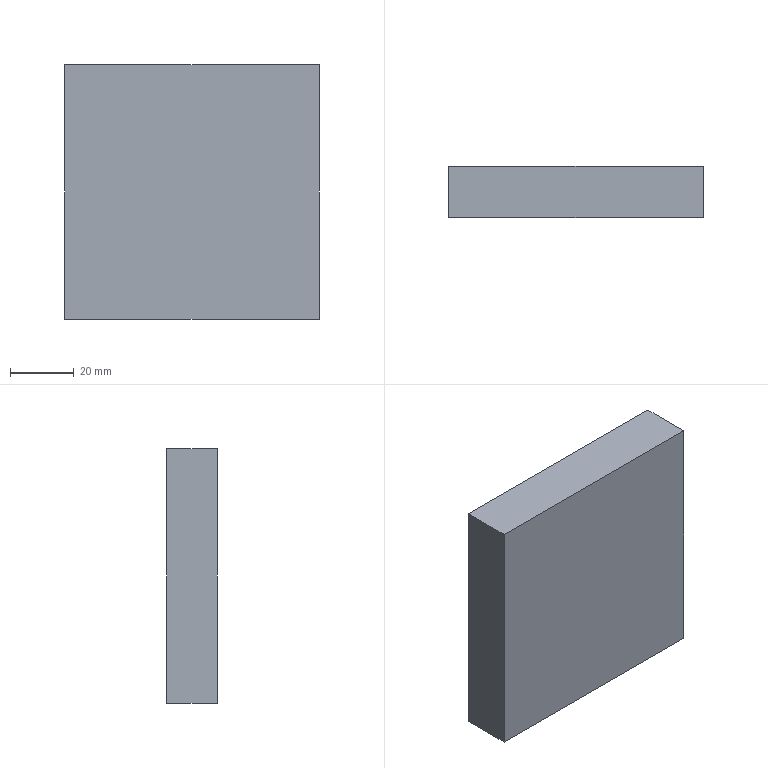Part | STEP file | HXGR200008-05-27 | 1 solid | 8 faces | box 80 x 16 x 80 mm | volume 101387 mm3 | plane 6 | cone 2
STEP:
#1=CARTESIAN_POINT('',(0.,8.008,0.));
#2=VERTEX_POINT('',#1);
#3=CARTESIAN_POINT('',(-11.,16.,0.));
#4=VERTEX_POINT('',#3);
#5=CARTESIAN_POINT('',(-11.,16.,0.));
#6=DIRECTION('',(-0.809,0.5878,0.));
#7=VECTOR('',#6,1000.);
#8=LINE('',#5,#7);
#9=EDGE_CURVE('',#2,#4,#8,.T.);
#10=ORIENTED_EDGE('',*,*,#9,.F.);
#11=CARTESIAN_POINT('',(11.,16.,0.));
#12=VERTEX_POINT('',#11);
#13=CARTESIAN_POINT('',(11.,16.,0.));
#14=DIRECTION('',(0.809,0.5878,0.));
#15=VECTOR('',#14,1000.);
#16=LINE('',#13,#15);
#17=EDGE_CURVE('',#2,#12,#16,.T.);
#18=ORIENTED_EDGE('',*,*,#17,.T.);
#19=CARTESIAN_POINT('',(0.,16.,0.));
#20=DIRECTION('',(0.,1.,0.));
#21=DIRECTION('',(-1.,0.,0.));
#22=AXIS2_PLACEMENT_3D('',#19,#20,#21);
#23=CIRCLE('',#22,11.);
#24=EDGE_CURVE('',#12,#4,#23,.T.);
#25=ORIENTED_EDGE('',*,*,#24,.T.);
#26=EDGE_LOOP('',(#10,#18,#25));
#27=FACE_OUTER_BOUND('',#26,.T.);
#28=CARTESIAN_POINT('',(0.,16.,0.));
#29=DIRECTION('',(0.,1.,0.));
#30=DIRECTION('',(-1.,0.,0.));
#31=AXIS2_PLACEMENT_3D('',#28,#29,#30);
#32=CONICAL_SURFACE('',#31,11.,0.9425);
#33=ADVANCED_FACE('',(#27),#32,.F.);
#34=CARTESIAN_POINT('',(-40.,0.,-40.));
#35=VERTEX_POINT('',#34);
#36=CARTESIAN_POINT('',(-40.,0.,40.));
#37=VERTEX_POINT('',#36);
#38=CARTESIAN_POINT('',(-40.,0.,40.));
#39=DIRECTION('',(0.,0.,1.));
#40=VECTOR('',#39,1000.);
#41=LINE('',#38,#40);
#42=EDGE_CURVE('',#35,#37,#41,.T.);
#43=ORIENTED_EDGE('',*,*,#42,.T.);
#44=CARTESIAN_POINT('',(-40.,16.,40.));
#45=VERTEX_POINT('',#44);
#46=CARTESIAN_POINT('',(-40.,16.,40.));
#47=DIRECTION('',(0.,-1.,0.));
#48=VECTOR('',#47,1000.);
#49=LINE('',#46,#48);
#50=EDGE_CURVE('',#45,#37,#49,.T.);
#51=ORIENTED_EDGE('',*,*,#50,.F.);
#52=CARTESIAN_POINT('',(-40.,16.,-40.));
#53=VERTEX_POINT('',#52);
#54=CARTESIAN_POINT('',(-40.,16.,40.));
#55=DIRECTION('',(0.,0.,1.));
#56=VECTOR('',#55,1000.);
#57=LINE('',#54,#56);
#58=EDGE_CURVE('',#53,#45,#57,.T.);
#59=ORIENTED_EDGE('',*,*,#58,.F.);
#60=CARTESIAN_POINT('',(-40.,16.,-40.));
#61=DIRECTION('',(0.,-1.,0.));
#62=VECTOR('',#61,1000.);
#63=LINE('',#60,#62);
#64=EDGE_CURVE('',#53,#35,#63,.T.);
#65=ORIENTED_EDGE('',*,*,#64,.T.);
#66=EDGE_LOOP('',(#43,#51,#59,#65));
#67=FACE_OUTER_BOUND('',#66,.T.);
#68=CARTESIAN_POINT('',(-40.,16.,40.));
#69=DIRECTION('',(1.,0.,0.));
#70=DIRECTION('',(0.,0.,-1.));
#71=AXIS2_PLACEMENT_3D('',#68,#69,#70);
#72=PLANE('',#71);
#73=ADVANCED_FACE('',(#67),#72,.F.);
#74=CARTESIAN_POINT('',(40.,0.,40.));
#75=VERTEX_POINT('',#74);
#76=CARTESIAN_POINT('',(40.,0.,40.));
#77=DIRECTION('',(1.,0.,0.));
#78=VECTOR('',#77,1000.);
#79=LINE('',#76,#78);
#80=EDGE_CURVE('',#37,#75,#79,.T.);
#81=ORIENTED_EDGE('',*,*,#80,.T.);
#82=CARTESIAN_POINT('',(40.,16.,40.));
#83=VERTEX_POINT('',#82);
#84=CARTESIAN_POINT('',(40.,16.,40.));
#85=DIRECTION('',(0.,-1.,0.));
#86=VECTOR('',#85,1000.);
#87=LINE('',#84,#86);
#88=EDGE_CURVE('',#83,#75,#87,.T.);
#89=ORIENTED_EDGE('',*,*,#88,.F.);
#90=CARTESIAN_POINT('',(40.,16.,40.));
#91=DIRECTION('',(1.,0.,0.));
#92=VECTOR('',#91,1000.);
#93=LINE('',#90,#92);
#94=EDGE_CURVE('',#45,#83,#93,.T.);
#95=ORIENTED_EDGE('',*,*,#94,.F.);
#96=ORIENTED_EDGE('',*,*,#50,.T.);
#97=EDGE_LOOP('',(#81,#89,#95,#96));
#98=FACE_OUTER_BOUND('',#97,.T.);
#99=CARTESIAN_POINT('',(40.,16.,40.));
#100=DIRECTION('',(0.,0.,-1.));
#101=DIRECTION('',(-1.,0.,0.));
#102=AXIS2_PLACEMENT_3D('',#99,#100,#101);
#103=PLANE('',#102);
#104=ADVANCED_FACE('',(#98),#103,.F.);
#105=CARTESIAN_POINT('',(40.,0.,-40.));
#106=VERTEX_POINT('',#105);
#107=CARTESIAN_POINT('',(40.,0.,40.));
#108=DIRECTION('',(0.,0.,-1.));
#109=VECTOR('',#108,1000.);
#110=LINE('',#107,#109);
#111=EDGE_CURVE('',#75,#106,#110,.T.);
#112=ORIENTED_EDGE('',*,*,#111,.T.);
#113=CARTESIAN_POINT('',(40.,16.,-40.));
#114=VERTEX_POINT('',#113);
#115=CARTESIAN_POINT('',(40.,16.,-40.));
#116=DIRECTION('',(0.,-1.,0.));
#117=VECTOR('',#116,1000.);
#118=LINE('',#115,#117);
#119=EDGE_CURVE('',#114,#106,#118,.T.);
#120=ORIENTED_EDGE('',*,*,#119,.F.);
#121=CARTESIAN_POINT('',(40.,16.,40.));
#122=DIRECTION('',(0.,0.,-1.));
#123=VECTOR('',#122,1000.);
#124=LINE('',#121,#123);
#125=EDGE_CURVE('',#83,#114,#124,.T.);
#126=ORIENTED_EDGE('',*,*,#125,.F.);
#127=ORIENTED_EDGE('',*,*,#88,.T.);
#128=EDGE_LOOP('',(#112,#120,#126,#127));
#129=FACE_OUTER_BOUND('',#128,.T.);
#130=CARTESIAN_POINT('',(40.,16.,40.));
#131=DIRECTION('',(-1.,0.,0.));
#132=DIRECTION('',(0.,0.,1.));
#133=AXIS2_PLACEMENT_3D('',#130,#131,#132);
#134=PLANE('',#133);
#135=ADVANCED_FACE('',(#129),#134,.F.);
#136=CARTESIAN_POINT('',(40.,0.,-40.));
#137=DIRECTION('',(-1.,0.,0.));
#138=VECTOR('',#137,1000.);
#139=LINE('',#136,#138);
#140=EDGE_CURVE('',#106,#35,#139,.T.);
#141=ORIENTED_EDGE('',*,*,#140,.T.);
#142=ORIENTED_EDGE('',*,*,#64,.F.);
#143=CARTESIAN_POINT('',(40.,16.,-40.));
#144=DIRECTION('',(-1.,0.,0.));
#145=VECTOR('',#144,1000.);
#146=LINE('',#143,#145);
#147=EDGE_CURVE('',#114,#53,#146,.T.);
#148=ORIENTED_EDGE('',*,*,#147,.F.);
#149=ORIENTED_EDGE('',*,*,#119,.T.);
#150=EDGE_LOOP('',(#141,#142,#148,#149));
#151=FACE_OUTER_BOUND('',#150,.T.);
#152=CARTESIAN_POINT('',(40.,16.,-40.));
#153=DIRECTION('',(0.,0.,1.));
#154=DIRECTION('',(1.,0.,0.));
#155=AXIS2_PLACEMENT_3D('',#152,#153,#154);
#156=PLANE('',#155);
#157=ADVANCED_FACE('',(#151),#156,.F.);
#158=CARTESIAN_POINT('',(0.,16.,0.));
#159=DIRECTION('',(0.,1.,0.));
#160=DIRECTION('',(-1.,0.,0.));
#161=AXIS2_PLACEMENT_3D('',#158,#159,#160);
#162=CIRCLE('',#161,11.);
#163=EDGE_CURVE('',#4,#12,#162,.T.);
#164=ORIENTED_EDGE('',*,*,#163,.F.);
#165=ORIENTED_EDGE('',*,*,#24,.F.);
#166=EDGE_LOOP('',(#164,#165));
#167=FACE_BOUND('',#166,.T.);
#168=ORIENTED_EDGE('',*,*,#58,.T.);
#169=ORIENTED_EDGE('',*,*,#94,.T.);
#170=ORIENTED_EDGE('',*,*,#125,.T.);
#171=ORIENTED_EDGE('',*,*,#147,.T.);
#172=EDGE_LOOP('',(#168,#169,#170,#171));
#173=FACE_OUTER_BOUND('',#172,.T.);
#174=CARTESIAN_POINT('',(0.,16.,0.));
#175=DIRECTION('',(0.,1.,0.));
#176=DIRECTION('',(0.,0.,1.));
#177=AXIS2_PLACEMENT_3D('',#174,#175,#176);
#178=PLANE('',#177);
#179=ADVANCED_FACE('',(#167,#173),#178,.T.);
#180=ORIENTED_EDGE('',*,*,#42,.F.);
#181=ORIENTED_EDGE('',*,*,#140,.F.);
#182=ORIENTED_EDGE('',*,*,#111,.F.);
#183=ORIENTED_EDGE('',*,*,#80,.F.);
#184=EDGE_LOOP('',(#180,#181,#182,#183));
#185=FACE_OUTER_BOUND('',#184,.T.);
#186=CARTESIAN_POINT('',(0.,0.,0.));
#187=DIRECTION('',(0.,1.,0.));
#188=DIRECTION('',(0.,0.,1.));
#189=AXIS2_PLACEMENT_3D('',#186,#187,#188);
#190=PLANE('',#189);
#191=ADVANCED_FACE('',(#185),#190,.F.);
#192=ORIENTED_EDGE('',*,*,#17,.F.);
#193=ORIENTED_EDGE('',*,*,#9,.T.);
#194=ORIENTED_EDGE('',*,*,#163,.T.);
#195=EDGE_LOOP('',(#192,#193,#194));
#196=FACE_OUTER_BOUND('',#195,.T.);
#197=CARTESIAN_POINT('',(0.,16.,0.));
#198=DIRECTION('',(0.,1.,0.));
#199=DIRECTION('',(-1.,0.,0.));
#200=AXIS2_PLACEMENT_3D('',#197,#198,#199);
#201=CONICAL_SURFACE('',#200,11.,0.9425);
#202=ADVANCED_FACE('',(#196),#201,.F.);
#203=CLOSED_SHELL('',(#33,#73,#104,#135,#157,#179,#191,#202));
#204=MANIFOLD_SOLID_BREP('',#203);
#205=CARTESIAN_POINT('',(0.,0.,0.));
#206=DIRECTION('',(0.,0.,1.));
#207=DIRECTION('',(1.,0.,0.));
#208=AXIS2_PLACEMENT_3D('',#205,#206,#207);
#209=(LENGTH_UNIT()NAMED_UNIT(*)SI_UNIT(.MILLI.,.METRE.));
#210=UNCERTAINTY_MEASURE_WITH_UNIT(LENGTH_MEASURE(0.00001),#209,'','');
#211=(NAMED_UNIT(*)PLANE_ANGLE_UNIT()SI_UNIT($,.RADIAN.));
#212=(NAMED_UNIT(*)SI_UNIT($,.STERADIAN.)SOLID_ANGLE_UNIT());
#213=(GEOMETRIC_REPRESENTATION_CONTEXT(3)GLOBAL_UNCERTAINTY_ASSIGNED_CONTEXT((#210))GLOBAL_UNIT_ASSIGNED_CONTEXT((#209,#211,#212))REPRESENTATION_CONTEXT('',''));
#214=ADVANCED_BREP_SHAPE_REPRESENTATION('',(#204,#208),#213);